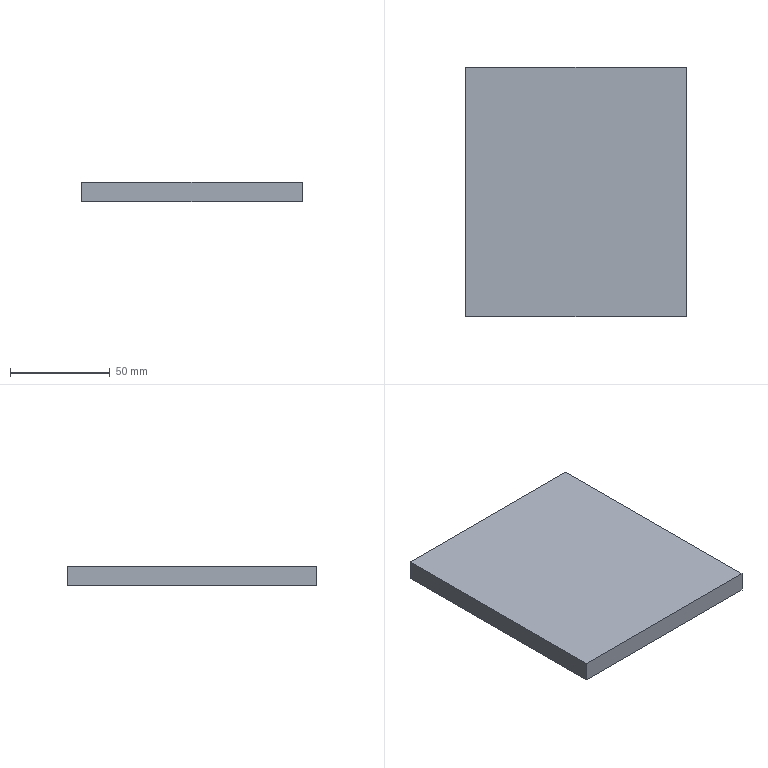Part | SolidWorks | features Extrusion 1 | 1 solid | 6 faces | box 110.487 x 124.868 x 10 mm | volume 137963 mm3 | plane 6
STEP:
#1=CARTESIAN_POINT('',(-55.984,63.789,0.));
#2=VERTEX_POINT('',#1);
#3=CARTESIAN_POINT('',(-55.984,-61.079,0.));
#4=VERTEX_POINT('',#3);
#5=CARTESIAN_POINT('',(-55.984,63.789,0.));
#6=DIRECTION('',(0.,-1.,0.));
#7=VECTOR('',#6,1000.);
#8=LINE('',#5,#7);
#9=EDGE_CURVE('',#2,#4,#8,.T.);
#10=ORIENTED_EDGE('',*,*,#9,.T.);
#11=CARTESIAN_POINT('',(-55.984,-61.079,10.));
#12=VERTEX_POINT('',#11);
#13=CARTESIAN_POINT('',(-55.984,-61.079,10.));
#14=DIRECTION('',(0.,0.,-1.));
#15=VECTOR('',#14,1000.);
#16=LINE('',#13,#15);
#17=EDGE_CURVE('',#12,#4,#16,.T.);
#18=ORIENTED_EDGE('',*,*,#17,.F.);
#19=CARTESIAN_POINT('',(-55.984,63.789,10.));
#20=VERTEX_POINT('',#19);
#21=CARTESIAN_POINT('',(-55.984,63.789,10.));
#22=DIRECTION('',(0.,-1.,0.));
#23=VECTOR('',#22,1000.);
#24=LINE('',#21,#23);
#25=EDGE_CURVE('',#20,#12,#24,.T.);
#26=ORIENTED_EDGE('',*,*,#25,.F.);
#27=CARTESIAN_POINT('',(-55.984,63.789,10.));
#28=DIRECTION('',(0.,0.,-1.));
#29=VECTOR('',#28,1000.);
#30=LINE('',#27,#29);
#31=EDGE_CURVE('',#20,#2,#30,.T.);
#32=ORIENTED_EDGE('',*,*,#31,.T.);
#33=EDGE_LOOP('',(#10,#18,#26,#32));
#34=FACE_OUTER_BOUND('',#33,.T.);
#35=CARTESIAN_POINT('',(-55.984,63.789,10.));
#36=DIRECTION('',(1.,0.,0.));
#37=DIRECTION('',(0.,0.,-1.));
#38=AXIS2_PLACEMENT_3D('',#35,#36,#37);
#39=PLANE('',#38);
#40=ADVANCED_FACE('',(#34),#39,.F.);
#41=CARTESIAN_POINT('',(54.503,-61.079,0.));
#42=VERTEX_POINT('',#41);
#43=CARTESIAN_POINT('',(-55.984,-61.079,0.));
#44=DIRECTION('',(1.,0.,0.));
#45=VECTOR('',#44,1000.);
#46=LINE('',#43,#45);
#47=EDGE_CURVE('',#4,#42,#46,.T.);
#48=ORIENTED_EDGE('',*,*,#47,.T.);
#49=CARTESIAN_POINT('',(54.503,-61.079,10.));
#50=VERTEX_POINT('',#49);
#51=CARTESIAN_POINT('',(54.503,-61.079,10.));
#52=DIRECTION('',(0.,0.,-1.));
#53=VECTOR('',#52,1000.);
#54=LINE('',#51,#53);
#55=EDGE_CURVE('',#50,#42,#54,.T.);
#56=ORIENTED_EDGE('',*,*,#55,.F.);
#57=CARTESIAN_POINT('',(-55.984,-61.079,10.));
#58=DIRECTION('',(1.,0.,0.));
#59=VECTOR('',#58,1000.);
#60=LINE('',#57,#59);
#61=EDGE_CURVE('',#12,#50,#60,.T.);
#62=ORIENTED_EDGE('',*,*,#61,.F.);
#63=ORIENTED_EDGE('',*,*,#17,.T.);
#64=EDGE_LOOP('',(#48,#56,#62,#63));
#65=FACE_OUTER_BOUND('',#64,.T.);
#66=CARTESIAN_POINT('',(-55.984,-61.079,10.));
#67=DIRECTION('',(0.,1.,0.));
#68=DIRECTION('',(0.,0.,1.));
#69=AXIS2_PLACEMENT_3D('',#66,#67,#68);
#70=PLANE('',#69);
#71=ADVANCED_FACE('',(#65),#70,.F.);
#72=CARTESIAN_POINT('',(54.503,63.789,0.));
#73=VERTEX_POINT('',#72);
#74=CARTESIAN_POINT('',(54.503,63.789,0.));
#75=DIRECTION('',(0.,1.,0.));
#76=VECTOR('',#75,1000.);
#77=LINE('',#74,#76);
#78=EDGE_CURVE('',#42,#73,#77,.T.);
#79=ORIENTED_EDGE('',*,*,#78,.T.);
#80=CARTESIAN_POINT('',(54.503,63.789,10.));
#81=VERTEX_POINT('',#80);
#82=CARTESIAN_POINT('',(54.503,63.789,10.));
#83=DIRECTION('',(0.,0.,-1.));
#84=VECTOR('',#83,1000.);
#85=LINE('',#82,#84);
#86=EDGE_CURVE('',#81,#73,#85,.T.);
#87=ORIENTED_EDGE('',*,*,#86,.F.);
#88=CARTESIAN_POINT('',(54.503,63.789,10.));
#89=DIRECTION('',(0.,1.,0.));
#90=VECTOR('',#89,1000.);
#91=LINE('',#88,#90);
#92=EDGE_CURVE('',#50,#81,#91,.T.);
#93=ORIENTED_EDGE('',*,*,#92,.F.);
#94=ORIENTED_EDGE('',*,*,#55,.T.);
#95=EDGE_LOOP('',(#79,#87,#93,#94));
#96=FACE_OUTER_BOUND('',#95,.T.);
#97=CARTESIAN_POINT('',(54.503,63.789,10.));
#98=DIRECTION('',(-1.,0.,0.));
#99=DIRECTION('',(0.,0.,1.));
#100=AXIS2_PLACEMENT_3D('',#97,#98,#99);
#101=PLANE('',#100);
#102=ADVANCED_FACE('',(#96),#101,.F.);
#103=CARTESIAN_POINT('',(-55.984,63.789,0.));
#104=DIRECTION('',(-1.,0.,0.));
#105=VECTOR('',#104,1000.);
#106=LINE('',#103,#105);
#107=EDGE_CURVE('',#73,#2,#106,.T.);
#108=ORIENTED_EDGE('',*,*,#107,.T.);
#109=ORIENTED_EDGE('',*,*,#31,.F.);
#110=CARTESIAN_POINT('',(-55.984,63.789,10.));
#111=DIRECTION('',(-1.,0.,0.));
#112=VECTOR('',#111,1000.);
#113=LINE('',#110,#112);
#114=EDGE_CURVE('',#81,#20,#113,.T.);
#115=ORIENTED_EDGE('',*,*,#114,.F.);
#116=ORIENTED_EDGE('',*,*,#86,.T.);
#117=EDGE_LOOP('',(#108,#109,#115,#116));
#118=FACE_OUTER_BOUND('',#117,.T.);
#119=CARTESIAN_POINT('',(-55.984,63.789,10.));
#120=DIRECTION('',(0.,-1.,0.));
#121=DIRECTION('',(0.,0.,-1.));
#122=AXIS2_PLACEMENT_3D('',#119,#120,#121);
#123=PLANE('',#122);
#124=ADVANCED_FACE('',(#118),#123,.F.);
#125=ORIENTED_EDGE('',*,*,#25,.T.);
#126=ORIENTED_EDGE('',*,*,#61,.T.);
#127=ORIENTED_EDGE('',*,*,#92,.T.);
#128=ORIENTED_EDGE('',*,*,#114,.T.);
#129=EDGE_LOOP('',(#125,#126,#127,#128));
#130=FACE_OUTER_BOUND('',#129,.T.);
#131=CARTESIAN_POINT('',(0.,0.,10.));
#132=DIRECTION('',(0.,0.,1.));
#133=DIRECTION('',(1.,0.,0.));
#134=AXIS2_PLACEMENT_3D('',#131,#132,#133);
#135=PLANE('',#134);
#136=ADVANCED_FACE('',(#130),#135,.T.);
#137=ORIENTED_EDGE('',*,*,#9,.F.);
#138=ORIENTED_EDGE('',*,*,#107,.F.);
#139=ORIENTED_EDGE('',*,*,#78,.F.);
#140=ORIENTED_EDGE('',*,*,#47,.F.);
#141=EDGE_LOOP('',(#137,#138,#139,#140));
#142=FACE_OUTER_BOUND('',#141,.T.);
#143=CARTESIAN_POINT('',(0.,0.,0.));
#144=DIRECTION('',(0.,0.,1.));
#145=DIRECTION('',(1.,0.,0.));
#146=AXIS2_PLACEMENT_3D('',#143,#144,#145);
#147=PLANE('',#146);
#148=ADVANCED_FACE('',(#142),#147,.F.);
#149=CLOSED_SHELL('',(#40,#71,#102,#124,#136,#148));
#150=MANIFOLD_SOLID_BREP('',#149);
#151=CARTESIAN_POINT('',(0.,0.,0.));
#152=DIRECTION('',(0.,0.,1.));
#153=DIRECTION('',(1.,0.,0.));
#154=AXIS2_PLACEMENT_3D('',#151,#152,#153);
#155=(LENGTH_UNIT()NAMED_UNIT(*)SI_UNIT(.MILLI.,.METRE.));
#156=UNCERTAINTY_MEASURE_WITH_UNIT(LENGTH_MEASURE(0.00001),#155,'','');
#157=(NAMED_UNIT(*)PLANE_ANGLE_UNIT()SI_UNIT($,.RADIAN.));
#158=(NAMED_UNIT(*)SI_UNIT($,.STERADIAN.)SOLID_ANGLE_UNIT());
#159=(GEOMETRIC_REPRESENTATION_CONTEXT(3)GLOBAL_UNCERTAINTY_ASSIGNED_CONTEXT((#156))GLOBAL_UNIT_ASSIGNED_CONTEXT((#155,#157,#158))REPRESENTATION_CONTEXT('',''));
#160=ADVANCED_BREP_SHAPE_REPRESENTATION('',(#150,#154),#159);